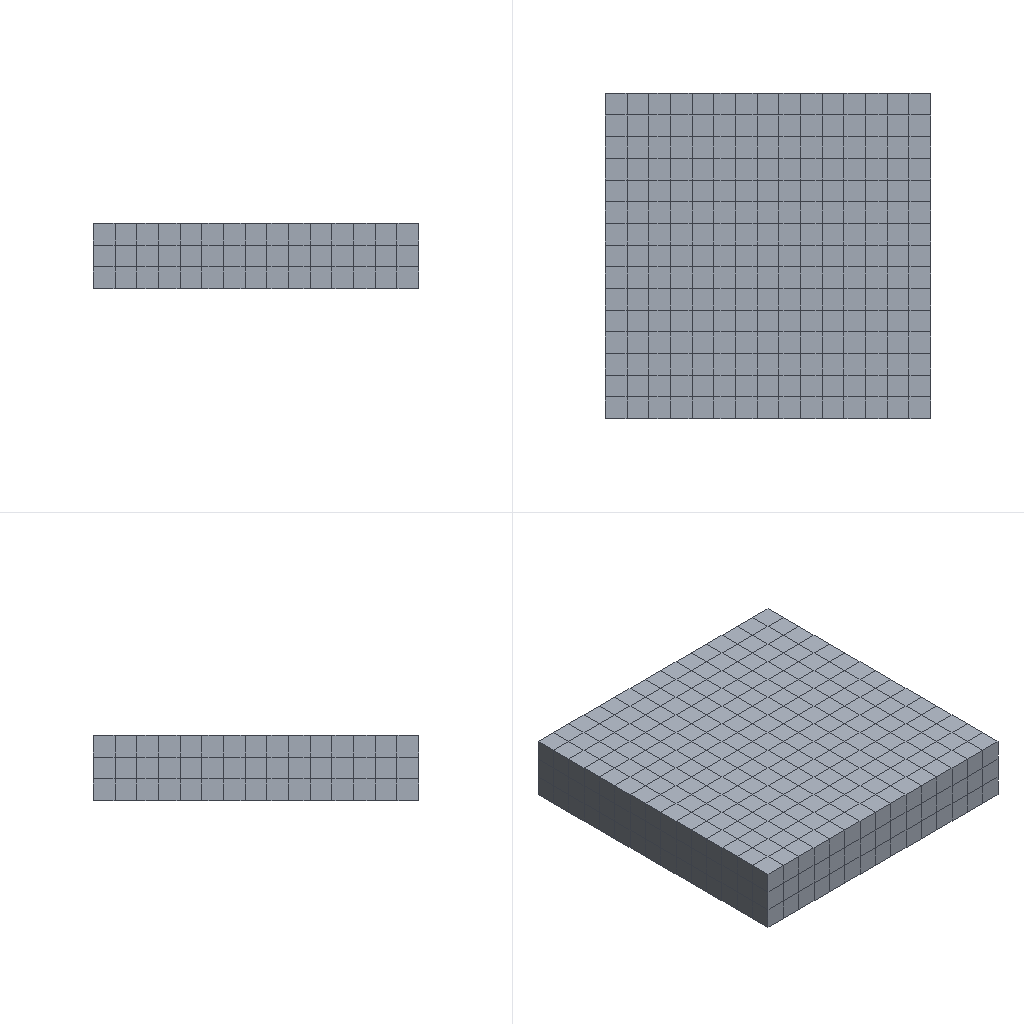Simulation study | ansys workbench
Ansys APDL input file, long lists of numbers shortened:
/batch
/config,noeldb,1     ! force off writing results to database
*get,_wallstrt,active,,time,wall
! ANSYS input file written by Workbench version 2022 R1
! File used for geometry attach:
/title,wbnew--____ (D5)
! ****** Begin Custom Load Command Snippet ******
/COM, ACT Extensions:
/COM,     LSDYNA, 2021.1
/COM,
! ****** End   Custom Load Command Snippet ******
*DIM,_wb_ProjectScratch_dir,string,248
_wb_ProjectScratch_dir(1) = ''
*DIM,_wb_SolverFiles_dir,string,248
_wb_SolverFiles_dir(1) = ''
*DIM,_wb_userfiles_dir,string,248
_wb_userfiles_dir(1) = ''
/com,--- Data in consistent NMM units. See Solving Units in the help system for more information.
/units,MPA
/nopr
/wb,file,start              !  signify a WB generated input file
/prep7
! Turn off shape checking because checks already performed inside WB mesher.
! See help system for more information.
SHPP,OFF,,NOWARN
/nolist
etcon,set             ! allow ANSYS to choose best KEYOP's for 180x elements, resets any applicable keyopt to MAPDL defaults
/com,*********** Nodes for the whole assembly ***********
nblock,3,,4083
(1i9,3e20.9e3)
        1    -2.166666667E+01     2.166666667E+01     3.333333333E+00
! (3711 more lines like these left out)
-1
/wb,elem,start            !  set before creation of elements
/com,*********** Elements for Body 1 "__12-FreeParts|____-____1" ***********
et,1,186
keyo,1,2,1          ! set full integration on SOLID186
eblock,19,solid,,675
(19i9)
        1        1        1        1        0        0        0        0       20        0        1        1      951      936      893      588      966      935      934
! (1349 more lines like these left out)
-1
/wb,elem,end               !  done creating elements
/com,*********** Send User Defined Coordinate System(s) ***********
csys,0
toffst,273.15,  ! Temperature offset from absolute zero
/com,*********** Set Reference Temperature ***********
tref,22.
/wb,mat,start              !  starting to send materials
/com,*********** Send Materials ***********
Temperature = 'TEMP' ! Temperature
MP,DENS,1,7.85e-09,	! tonne mm^-3
MP,ALPX,1,1.2e-05,	! C^-1
MP,C,1,434000000,	! mm^2 s^-2 C^-1
MP,KXX,1,60.5,	! tonne mm s^-3 C^-1
MP,RSVX,1,0.00017,	! ohm mm
MP,EX,1,200000,	! tonne s^-2 mm^-1
MP,NUXY,1,0.3,
MP,MURX,1,10000,
/wb,mat,end                !  done sending materials
!************************* Model Summary ********************
!__12-FreeParts|____-____1,	结构钢,	matid,	1
!************************* End Model Summary ********************
! get the diagonal of the bounding box. Needed later for other things
*get,_xmin,node,,mnloc,x
*get,_ymin,node,,mnloc,y
*get,_zmin,node,,mnloc,z
*get,_xmax,node,,mxloc,x
*get,_ymax,node,,mxloc,y
*get,_zmax,node,,mxloc,z
_ASMDIAG=(_xmax-_xmin)*(_xmax-_xmin)+(_ymax-_ymin)*(_ymax-_ymin)+(_zmax-_zmin)*(_zmax-_zmin)
_ASMDIAG=SQRT(_ASMDIAG)
/wb,contact,start          !  starting to send contact
/wb,contact,end            !  done creating contacts
/golist
/wb,load,start             !  starting to send loads
/com,*********** Fixed Supports ***********
CMBLOCK,_FIXEDSU,NODE,      172
(8i10)
       799       800       801       802       803       804       805       806
! (21 more lines like these left out)
cmsel,s,_FIXEDSU
d,all,all
nsel,all
/com,*********** Define Pressure Using Surface Effect Elements "__" ***********
et,2,154
eblock,10,,,45
(15i9)
     1306        2        2        2        0      936      893      934      935     3499     3498     3565     3566
! (44 more lines like these left out)
-1
esel,s,type,,2
keyop,2,7,0                ! Use deformed area for application of load
esel,all
/com,*********** Define Pressure Using Surface Effect Elements "__ 2" ***********
et,3,154
eblock,10,,,45
(15i9)
     1351        3        3        3        0      982      983      798      799     3645     3321     3320     3323
! (44 more lines like these left out)
-1
esel,s,type,,3
keyop,3,7,0                ! Use deformed area for application of load
esel,all
esel,all
/gst,on,on
fini
*get,_numnode,node,0,count
*get,_numelem,elem,0,count
*get, _MAXELEMNUM, elem, 0, NUM, MAX
*get, _MAXNODENUM, node, 0, NUM, MAX
*get, _MAXELEMTYPE, etyp, 0, NUM, MAX
*get, _MAXREALCONST, real, 0, NUM, MAX
/go
/wb,load,end               !  done creating loads
/com,--- Number of total nodes = %_numnode%
/com,--- Number of contact elements = 90
/com,--- Number of spring elements = 0
/com,--- Number of bearing elements = 0
/com,--- Number of solid elements = 675
/com,--- Number of condensed parts = 0
/com,--- Number of total elements = %_numelem%
*get,_wallbsol,active,,time,wall
/com,****************************************************************************
/com,*************************    SOLUTION       ********************************
/com,****************************************************************************
/solu
antype,0                   ! static analysis
_thickRatio=  1     ! Ratio of thick parts in the model
eqsl,pcg,1e-8,,,,,,1
cntr,print,1               ! print out contact info and also make no initial contact an error
dmpoption,emat,no             ! Don't combine emat file for DANSYS
dmpoption,esav,no             ! Don't combine esav file for DANSYS
nldiag,cont,iter           ! print out contact info each equilibrium iteration
rescontrol,,none                 ! Do not keep any restart files
/com,****************************************************
/com,******************* SOLVE FOR LS 1 OF 1 ****************
esel,s,type,,2
nsle
sf,all,pres,-100.
esel,s,type,,3
nsle
sf,all,pres,-100.
nsel,all
esel,all
esel,all
/nopr
/gopr
nsub,1,1,1
time,1.
outres,erase
outres,all,none
outres,nsol,all,
outres,rsol,all
outres,eangl,all
outres,etmp,all
outres,veng,all
outres,strs,all,
outres,epel,all,
outres,eppl,all,
outres,cont,all,
! *********** WB SOLVE COMMAND ***********
! check interactive state
*get,ANSINTER_,active,,int
*if,ANSINTER_,ne,0,then
/eof
*endif
solve
/com *************** Write FE CONNECTORS *********
CEWRITE,file,ce,,INTE
/com,****************************************************
/com,*************** FINISHED SOLVE FOR LS 1 *************
*get,_wallasol,active,,time,wall
/nopr
*get,_numnode,node,0,count
*get,_numelem,elem,0,count
*get, _MAXELEMNUM, elem, 0, NUM, MAX
*get, _MAXNODENUM, node, 0, NUM, MAX,,,INTERNAL
*get, _MAXELEMTYPE, etyp, 0, NUM, MAX
*get, _MAXREALCONST, real, 0, NUM, MAX
/gopr
*get,_PCGITER,active,,solu,cgiter
/post1
xmlo,ENCODING,ISO-8859-1
xmlo,parm
/xml,parm,xml
fini
/gopr
*get,_walldone,active,,time,wall
_preptime=(_wallbsol-_wallstrt)*3600
_solvtime=(_wallasol-_wallbsol)*3600
_posttime=(_walldone-_wallasol)*3600
_totaltim=(_walldone-_wallstrt)*3600
*get,_dlbratio,active,0,solu,dlbr
*get,_combtime,active,0,solu,comb
*get,_ssmode,active,0,solu,ssmm
*get,_ndofs,active,0,solu,ndof
*get,_sol_end_time,active,0,set,time
*if,_sol_end_time,eq,1.,then
/fclean				!clean distributed files
*endif
/com,--- Total number of nodes = %_numnode%
/com,--- Total number of elements = %_numelem%
/com,--- Element load balance ratio = %_dlbratio%
/com,--- Time to combine distributed files = %_combtime%
/com,--- Sparse memory mode = %_ssmode%
/com,--- Number of DOF = %_ndofs%
/wb,file,end               ! done with WB generated input